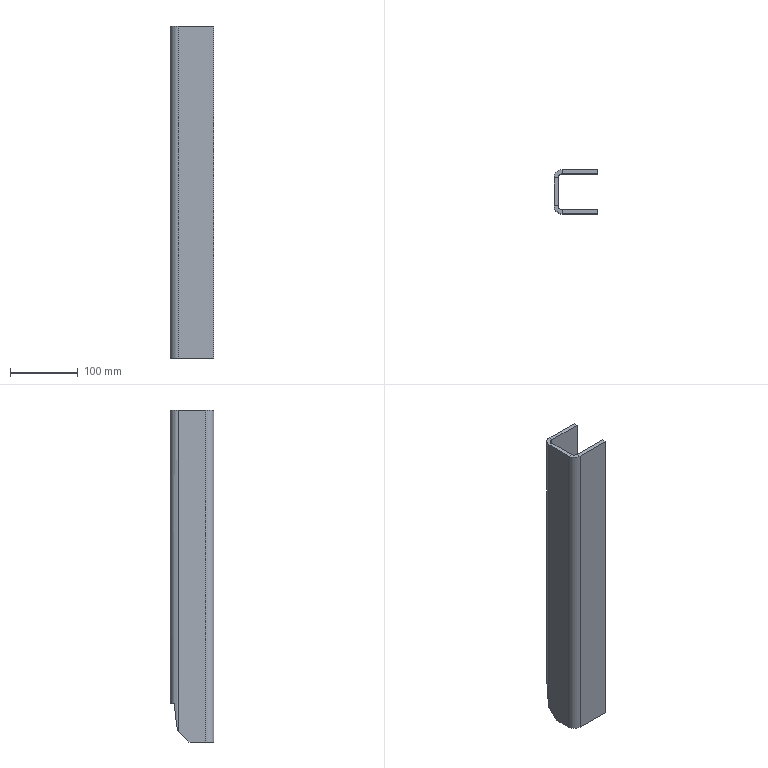Part | STEP file | 11-Bent plate | 1 solid | 23 faces | box 65 x 65 x 491 mm | volume 493529 mm3 | plane 19 | cylinder 4 | commonest cylinder face diameters 12 x2 24 x2